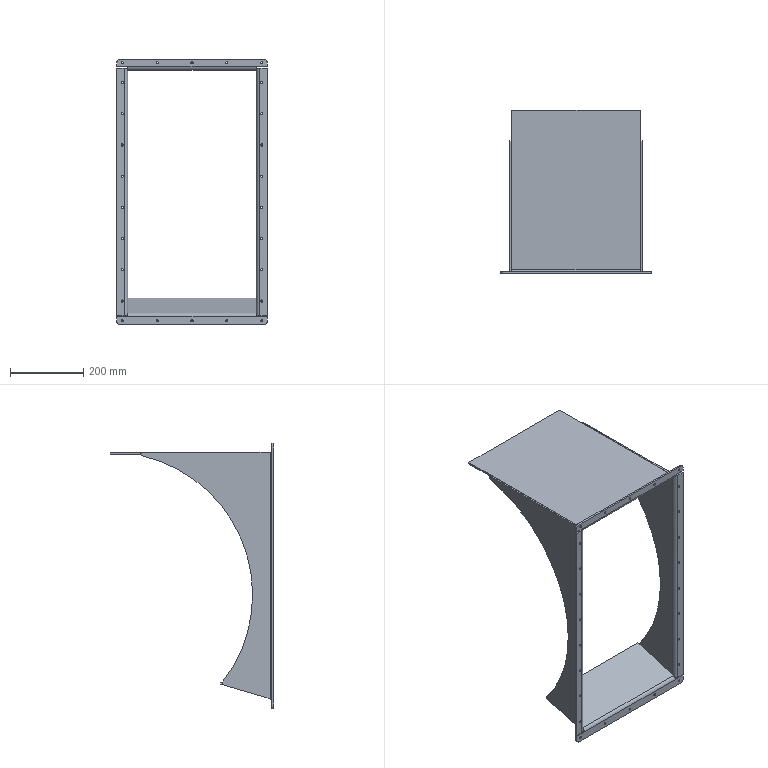Part | SolidWorks | 4 solids | 172 faces | box 410 x 445 x 723.639 mm | volume 2057835 mm3 | cylinder 70 | cone 52 | plane 48 | spline 2 | commonest cylinder face diameters 6 x52 10 x8 20 x8 775 x2